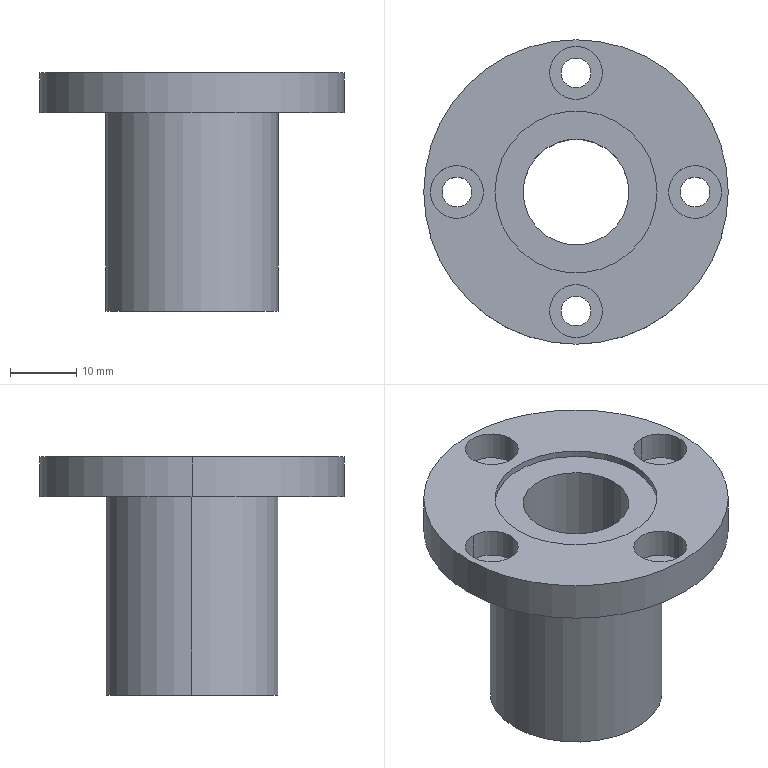Part | SolidWorks | features BaseBody 1 | 1 solid | 35 faces | box 46 x 46 x 36 mm | volume 17134 mm3 | cylinder 26 | plane 9 | commonest cylinder face diameters 4.5 x8 8 x8 24.5 x4 16 x2 26 x2 46 x2
STEP:
#1=CARTESIAN_POINT('',(13.,0.,-18.));
#2=VERTEX_POINT('',#1);
#3=CARTESIAN_POINT('',(-13.,0.,-18.));
#4=VERTEX_POINT('',#3);
#5=CARTESIAN_POINT('',(0.,0.,-18.));
#6=DIRECTION('',(0.,0.,1.));
#7=DIRECTION('',(1.,0.,0.));
#8=AXIS2_PLACEMENT_3D('',#5,#6,#7);
#9=CIRCLE('',#8,13.);
#10=EDGE_CURVE('',#2,#4,#9,.T.);
#11=ORIENTED_EDGE('',*,*,#10,.T.);
#12=CARTESIAN_POINT('',(-13.,0.,12.));
#13=VERTEX_POINT('',#12);
#14=CARTESIAN_POINT('',(-13.,0.,0.));
#15=DIRECTION('',(0.,0.,1.));
#16=VECTOR('',#15,1000.);
#17=LINE('',#14,#16);
#18=EDGE_CURVE('',#4,#13,#17,.T.);
#19=ORIENTED_EDGE('',*,*,#18,.T.);
#20=CARTESIAN_POINT('',(13.,0.,12.));
#21=VERTEX_POINT('',#20);
#22=CARTESIAN_POINT('',(0.,0.,12.));
#23=DIRECTION('',(0.,0.,-1.));
#24=DIRECTION('',(1.,0.,0.));
#25=AXIS2_PLACEMENT_3D('',#22,#23,#24);
#26=CIRCLE('',#25,13.);
#27=EDGE_CURVE('',#13,#21,#26,.T.);
#28=ORIENTED_EDGE('',*,*,#27,.T.);
#29=CARTESIAN_POINT('',(13.,0.,0.));
#30=DIRECTION('',(0.,0.,1.));
#31=VECTOR('',#30,1000.);
#32=LINE('',#29,#31);
#33=EDGE_CURVE('',#2,#21,#32,.T.);
#34=ORIENTED_EDGE('',*,*,#33,.F.);
#35=EDGE_LOOP('',(#11,#19,#28,#34));
#36=FACE_OUTER_BOUND('',#35,.T.);
#37=CARTESIAN_POINT('',(0.,0.,0.));
#38=DIRECTION('',(0.,0.,1.));
#39=DIRECTION('',(1.,0.,0.));
#40=AXIS2_PLACEMENT_3D('',#37,#38,#39);
#41=CYLINDRICAL_SURFACE('',#40,13.);
#42=ADVANCED_FACE('',(#36),#41,.T.);
#43=CARTESIAN_POINT('',(18.,-2.25,13.6));
#44=VERTEX_POINT('',#43);
#45=CARTESIAN_POINT('',(18.,2.25,13.6));
#46=VERTEX_POINT('',#45);
#47=CARTESIAN_POINT('',(18.,0.,13.6));
#48=DIRECTION('',(0.,0.,-1.));
#49=DIRECTION('',(0.,1.,0.));
#50=AXIS2_PLACEMENT_3D('',#47,#48,#49);
#51=CIRCLE('',#50,2.25);
#52=EDGE_CURVE('',#44,#46,#51,.T.);
#53=ORIENTED_EDGE('',*,*,#52,.F.);
#54=CARTESIAN_POINT('',(18.,-2.25,12.));
#55=VERTEX_POINT('',#54);
#56=CARTESIAN_POINT('',(18.,-2.25,13.6));
#57=DIRECTION('',(0.,0.,-1.));
#58=VECTOR('',#57,1000.);
#59=LINE('',#56,#58);
#60=EDGE_CURVE('',#44,#55,#59,.T.);
#61=ORIENTED_EDGE('',*,*,#60,.T.);
#62=CARTESIAN_POINT('',(18.,2.25,12.));
#63=VERTEX_POINT('',#62);
#64=CARTESIAN_POINT('',(18.,0.,12.));
#65=DIRECTION('',(0.,0.,1.));
#66=DIRECTION('',(0.,1.,0.));
#67=AXIS2_PLACEMENT_3D('',#64,#65,#66);
#68=CIRCLE('',#67,2.25);
#69=EDGE_CURVE('',#63,#55,#68,.T.);
#70=ORIENTED_EDGE('',*,*,#69,.F.);
#71=CARTESIAN_POINT('',(18.,2.25,13.6));
#72=DIRECTION('',(0.,0.,-1.));
#73=VECTOR('',#72,1000.);
#74=LINE('',#71,#73);
#75=EDGE_CURVE('',#46,#63,#74,.T.);
#76=ORIENTED_EDGE('',*,*,#75,.F.);
#77=EDGE_LOOP('',(#53,#61,#70,#76));
#78=FACE_OUTER_BOUND('',#77,.T.);
#79=CARTESIAN_POINT('',(18.,0.,13.6));
#80=DIRECTION('',(0.,0.,-1.));
#81=DIRECTION('',(0.,1.,0.));
#82=AXIS2_PLACEMENT_3D('',#79,#80,#81);
#83=CYLINDRICAL_SURFACE('',#82,2.25);
#84=ADVANCED_FACE('',(#78),#83,.F.);
#85=CARTESIAN_POINT('',(2.25,18.,13.6));
#86=VERTEX_POINT('',#85);
#87=CARTESIAN_POINT('',(-2.25,18.,13.6));
#88=VERTEX_POINT('',#87);
#89=CARTESIAN_POINT('',(0.,18.,13.6));
#90=DIRECTION('',(0.,0.,-1.));
#91=DIRECTION('',(-1.,0.,0.));
#92=AXIS2_PLACEMENT_3D('',#89,#90,#91);
#93=CIRCLE('',#92,2.25);
#94=EDGE_CURVE('',#86,#88,#93,.T.);
#95=ORIENTED_EDGE('',*,*,#94,.F.);
#96=CARTESIAN_POINT('',(2.25,18.,12.));
#97=VERTEX_POINT('',#96);
#98=CARTESIAN_POINT('',(2.25,18.,13.6));
#99=DIRECTION('',(0.,0.,-1.));
#100=VECTOR('',#99,1000.);
#101=LINE('',#98,#100);
#102=EDGE_CURVE('',#86,#97,#101,.T.);
#103=ORIENTED_EDGE('',*,*,#102,.T.);
#104=CARTESIAN_POINT('',(-2.25,18.,12.));
#105=VERTEX_POINT('',#104);
#106=CARTESIAN_POINT('',(0.,18.,12.));
#107=DIRECTION('',(0.,0.,1.));
#108=DIRECTION('',(-1.,0.,0.));
#109=AXIS2_PLACEMENT_3D('',#106,#107,#108);
#110=CIRCLE('',#109,2.25);
#111=EDGE_CURVE('',#105,#97,#110,.T.);
#112=ORIENTED_EDGE('',*,*,#111,.F.);
#113=CARTESIAN_POINT('',(-2.25,18.,13.6));
#114=DIRECTION('',(0.,0.,-1.));
#115=VECTOR('',#114,1000.);
#116=LINE('',#113,#115);
#117=EDGE_CURVE('',#88,#105,#116,.T.);
#118=ORIENTED_EDGE('',*,*,#117,.F.);
#119=EDGE_LOOP('',(#95,#103,#112,#118));
#120=FACE_OUTER_BOUND('',#119,.T.);
#121=CARTESIAN_POINT('',(0.,18.,13.6));
#122=DIRECTION('',(0.,0.,-1.));
#123=DIRECTION('',(-1.,0.,0.));
#124=AXIS2_PLACEMENT_3D('',#121,#122,#123);
#125=CYLINDRICAL_SURFACE('',#124,2.25);
#126=ADVANCED_FACE('',(#120),#125,.F.);
#127=CARTESIAN_POINT('',(-18.,-2.25,13.6));
#128=VERTEX_POINT('',#127);
#129=CARTESIAN_POINT('',(-18.,2.25,13.6));
#130=VERTEX_POINT('',#129);
#131=CARTESIAN_POINT('',(-18.,0.,13.6));
#132=DIRECTION('',(0.,0.,-1.));
#133=DIRECTION('',(0.,1.,0.));
#134=AXIS2_PLACEMENT_3D('',#131,#132,#133);
#135=CIRCLE('',#134,2.25);
#136=EDGE_CURVE('',#128,#130,#135,.T.);
#137=ORIENTED_EDGE('',*,*,#136,.F.);
#138=CARTESIAN_POINT('',(-18.,-2.25,12.));
#139=VERTEX_POINT('',#138);
#140=CARTESIAN_POINT('',(-18.,-2.25,13.6));
#141=DIRECTION('',(0.,0.,-1.));
#142=VECTOR('',#141,1000.);
#143=LINE('',#140,#142);
#144=EDGE_CURVE('',#128,#139,#143,.T.);
#145=ORIENTED_EDGE('',*,*,#144,.T.);
#146=CARTESIAN_POINT('',(-18.,2.25,12.));
#147=VERTEX_POINT('',#146);
#148=CARTESIAN_POINT('',(-18.,0.,12.));
#149=DIRECTION('',(0.,0.,1.));
#150=DIRECTION('',(0.,1.,0.));
#151=AXIS2_PLACEMENT_3D('',#148,#149,#150);
#152=CIRCLE('',#151,2.25);
#153=EDGE_CURVE('',#147,#139,#152,.T.);
#154=ORIENTED_EDGE('',*,*,#153,.F.);
#155=CARTESIAN_POINT('',(-18.,2.25,13.6));
#156=DIRECTION('',(0.,0.,-1.));
#157=VECTOR('',#156,1000.);
#158=LINE('',#155,#157);
#159=EDGE_CURVE('',#130,#147,#158,.T.);
#160=ORIENTED_EDGE('',*,*,#159,.F.);
#161=EDGE_LOOP('',(#137,#145,#154,#160));
#162=FACE_OUTER_BOUND('',#161,.T.);
#163=CARTESIAN_POINT('',(-18.,0.,13.6));
#164=DIRECTION('',(0.,0.,-1.));
#165=DIRECTION('',(0.,1.,0.));
#166=AXIS2_PLACEMENT_3D('',#163,#164,#165);
#167=CYLINDRICAL_SURFACE('',#166,2.25);
#168=ADVANCED_FACE('',(#162),#167,.F.);
#169=CARTESIAN_POINT('',(2.25,-18.,13.6));
#170=VERTEX_POINT('',#169);
#171=CARTESIAN_POINT('',(-2.25,-18.,13.6));
#172=VERTEX_POINT('',#171);
#173=CARTESIAN_POINT('',(0.,-18.,13.6));
#174=DIRECTION('',(0.,0.,-1.));
#175=DIRECTION('',(-1.,0.,0.));
#176=AXIS2_PLACEMENT_3D('',#173,#174,#175);
#177=CIRCLE('',#176,2.25);
#178=EDGE_CURVE('',#170,#172,#177,.T.);
#179=ORIENTED_EDGE('',*,*,#178,.F.);
#180=CARTESIAN_POINT('',(2.25,-18.,12.));
#181=VERTEX_POINT('',#180);
#182=CARTESIAN_POINT('',(2.25,-18.,13.6));
#183=DIRECTION('',(0.,0.,-1.));
#184=VECTOR('',#183,1000.);
#185=LINE('',#182,#184);
#186=EDGE_CURVE('',#170,#181,#185,.T.);
#187=ORIENTED_EDGE('',*,*,#186,.T.);
#188=CARTESIAN_POINT('',(-2.25,-18.,12.));
#189=VERTEX_POINT('',#188);
#190=CARTESIAN_POINT('',(0.,-18.,12.));
#191=DIRECTION('',(0.,0.,1.));
#192=DIRECTION('',(-1.,0.,0.));
#193=AXIS2_PLACEMENT_3D('',#190,#191,#192);
#194=CIRCLE('',#193,2.25);
#195=EDGE_CURVE('',#189,#181,#194,.T.);
#196=ORIENTED_EDGE('',*,*,#195,.F.);
#197=CARTESIAN_POINT('',(-2.25,-18.,13.6));
#198=DIRECTION('',(0.,0.,-1.));
#199=VECTOR('',#198,1000.);
#200=LINE('',#197,#199);
#201=EDGE_CURVE('',#172,#189,#200,.T.);
#202=ORIENTED_EDGE('',*,*,#201,.F.);
#203=EDGE_LOOP('',(#179,#187,#196,#202));
#204=FACE_OUTER_BOUND('',#203,.T.);
#205=CARTESIAN_POINT('',(0.,-18.,13.6));
#206=DIRECTION('',(0.,0.,-1.));
#207=DIRECTION('',(-1.,0.,0.));
#208=AXIS2_PLACEMENT_3D('',#205,#206,#207);
#209=CYLINDRICAL_SURFACE('',#208,2.25);
#210=ADVANCED_FACE('',(#204),#209,.F.);
#211=CARTESIAN_POINT('',(-23.,0.,18.));
#212=VERTEX_POINT('',#211);
#213=CARTESIAN_POINT('',(23.,0.,18.));
#214=VERTEX_POINT('',#213);
#215=CARTESIAN_POINT('',(0.,0.,18.));
#216=DIRECTION('',(0.,0.,-1.));
#217=DIRECTION('',(-1.,0.,0.));
#218=AXIS2_PLACEMENT_3D('',#215,#216,#217);
#219=CIRCLE('',#218,23.);
#220=EDGE_CURVE('',#212,#214,#219,.T.);
#221=ORIENTED_EDGE('',*,*,#220,.T.);
#222=CARTESIAN_POINT('',(23.,0.,12.));
#223=VERTEX_POINT('',#222);
#224=CARTESIAN_POINT('',(23.,0.,18.));
#225=DIRECTION('',(0.,0.,-1.));
#226=VECTOR('',#225,1000.);
#227=LINE('',#224,#226);
#228=EDGE_CURVE('',#214,#223,#227,.T.);
#229=ORIENTED_EDGE('',*,*,#228,.T.);
#230=CARTESIAN_POINT('',(-23.,0.,12.));
#231=VERTEX_POINT('',#230);
#232=CARTESIAN_POINT('',(0.,0.,12.));
#233=DIRECTION('',(0.,0.,-1.));
#234=DIRECTION('',(-1.,0.,0.));
#235=AXIS2_PLACEMENT_3D('',#232,#233,#234);
#236=CIRCLE('',#235,23.);
#237=EDGE_CURVE('',#231,#223,#236,.T.);
#238=ORIENTED_EDGE('',*,*,#237,.F.);
#239=CARTESIAN_POINT('',(-23.,0.,18.));
#240=DIRECTION('',(0.,0.,-1.));
#241=VECTOR('',#240,1000.);
#242=LINE('',#239,#241);
#243=EDGE_CURVE('',#212,#231,#242,.T.);
#244=ORIENTED_EDGE('',*,*,#243,.F.);
#245=EDGE_LOOP('',(#221,#229,#238,#244));
#246=FACE_OUTER_BOUND('',#245,.T.);
#247=CARTESIAN_POINT('',(0.,0.,18.));
#248=DIRECTION('',(0.,0.,-1.));
#249=DIRECTION('',(-1.,0.,0.));
#250=AXIS2_PLACEMENT_3D('',#247,#248,#249);
#251=CYLINDRICAL_SURFACE('',#250,23.);
#252=ADVANCED_FACE('',(#246),#251,.T.);
#253=CARTESIAN_POINT('',(-12.25,0.,-18.));
#254=VERTEX_POINT('',#253);
#255=CARTESIAN_POINT('',(12.25,0.,-18.));
#256=VERTEX_POINT('',#255);
#257=CARTESIAN_POINT('',(0.,0.,-18.));
#258=DIRECTION('',(0.,0.,1.));
#259=DIRECTION('',(1.,0.,0.));
#260=AXIS2_PLACEMENT_3D('',#257,#258,#259);
#261=CIRCLE('',#260,12.25);
#262=EDGE_CURVE('',#254,#256,#261,.T.);
#263=ORIENTED_EDGE('',*,*,#262,.F.);
#264=CARTESIAN_POINT('',(-12.25,0.,-17.));
#265=VERTEX_POINT('',#264);
#266=CARTESIAN_POINT('',(-12.25,0.,0.));
#267=DIRECTION('',(0.,0.,1.));
#268=VECTOR('',#267,1000.);
#269=LINE('',#266,#268);
#270=EDGE_CURVE('',#254,#265,#269,.T.);
#271=ORIENTED_EDGE('',*,*,#270,.T.);
#272=CARTESIAN_POINT('',(12.25,0.,-17.));
#273=VERTEX_POINT('',#272);
#274=CARTESIAN_POINT('',(0.,0.,-17.));
#275=DIRECTION('',(0.,0.,-1.));
#276=DIRECTION('',(1.,0.,0.));
#277=AXIS2_PLACEMENT_3D('',#274,#275,#276);
#278=CIRCLE('',#277,12.25);
#279=EDGE_CURVE('',#273,#265,#278,.T.);
#280=ORIENTED_EDGE('',*,*,#279,.F.);
#281=CARTESIAN_POINT('',(12.25,0.,0.));
#282=DIRECTION('',(0.,0.,1.));
#283=VECTOR('',#282,1000.);
#284=LINE('',#281,#283);
#285=EDGE_CURVE('',#256,#273,#284,.T.);
#286=ORIENTED_EDGE('',*,*,#285,.F.);
#287=EDGE_LOOP('',(#263,#271,#280,#286));
#288=FACE_OUTER_BOUND('',#287,.T.);
#289=CARTESIAN_POINT('',(0.,0.,0.));
#290=DIRECTION('',(0.,0.,1.));
#291=DIRECTION('',(1.,0.,0.));
#292=AXIS2_PLACEMENT_3D('',#289,#290,#291);
#293=CYLINDRICAL_SURFACE('',#292,12.25);
#294=ADVANCED_FACE('',(#288),#293,.F.);
#295=CARTESIAN_POINT('',(18.,4.,18.));
#296=VERTEX_POINT('',#295);
#297=CARTESIAN_POINT('',(18.,-4.,18.));
#298=VERTEX_POINT('',#297);
#299=CARTESIAN_POINT('',(18.,0.,18.));
#300=DIRECTION('',(0.,0.,1.));
#301=DIRECTION('',(0.,1.,0.));
#302=AXIS2_PLACEMENT_3D('',#299,#300,#301);
#303=CIRCLE('',#302,4.);
#304=EDGE_CURVE('',#296,#298,#303,.T.);
#305=ORIENTED_EDGE('',*,*,#304,.T.);
#306=CARTESIAN_POINT('',(18.,-4.,13.6));
#307=VERTEX_POINT('',#306);
#308=CARTESIAN_POINT('',(18.,-4.,18.));
#309=DIRECTION('',(0.,0.,-1.));
#310=VECTOR('',#309,1000.);
#311=LINE('',#308,#310);
#312=EDGE_CURVE('',#298,#307,#311,.T.);
#313=ORIENTED_EDGE('',*,*,#312,.T.);
#314=CARTESIAN_POINT('',(18.,4.,13.6));
#315=VERTEX_POINT('',#314);
#316=CARTESIAN_POINT('',(18.,0.,13.6));
#317=DIRECTION('',(0.,0.,-1.));
#318=DIRECTION('',(0.,1.,0.));
#319=AXIS2_PLACEMENT_3D('',#316,#317,#318);
#320=CIRCLE('',#319,4.);
#321=EDGE_CURVE('',#307,#315,#320,.T.);
#322=ORIENTED_EDGE('',*,*,#321,.T.);
#323=CARTESIAN_POINT('',(18.,4.,18.));
#324=DIRECTION('',(0.,0.,-1.));
#325=VECTOR('',#324,1000.);
#326=LINE('',#323,#325);
#327=EDGE_CURVE('',#296,#315,#326,.T.);
#328=ORIENTED_EDGE('',*,*,#327,.F.);
#329=EDGE_LOOP('',(#305,#313,#322,#328));
#330=FACE_OUTER_BOUND('',#329,.T.);
#331=CARTESIAN_POINT('',(18.,0.,18.));
#332=DIRECTION('',(0.,0.,-1.));
#333=DIRECTION('',(0.,1.,0.));
#334=AXIS2_PLACEMENT_3D('',#331,#332,#333);
#335=CYLINDRICAL_SURFACE('',#334,4.);
#336=ADVANCED_FACE('',(#330),#335,.F.);
#337=CARTESIAN_POINT('',(-4.,18.,18.));
#338=VERTEX_POINT('',#337);
#339=CARTESIAN_POINT('',(4.,18.,18.));
#340=VERTEX_POINT('',#339);
#341=CARTESIAN_POINT('',(0.,18.,18.));
#342=DIRECTION('',(0.,0.,1.));
#343=DIRECTION('',(-1.,0.,0.));
#344=AXIS2_PLACEMENT_3D('',#341,#342,#343);
#345=CIRCLE('',#344,4.);
#346=EDGE_CURVE('',#338,#340,#345,.T.);
#347=ORIENTED_EDGE('',*,*,#346,.T.);
#348=CARTESIAN_POINT('',(4.,18.,13.6));
#349=VERTEX_POINT('',#348);
#350=CARTESIAN_POINT('',(4.,18.,18.));
#351=DIRECTION('',(0.,0.,-1.));
#352=VECTOR('',#351,1000.);
#353=LINE('',#350,#352);
#354=EDGE_CURVE('',#340,#349,#353,.T.);
#355=ORIENTED_EDGE('',*,*,#354,.T.);
#356=CARTESIAN_POINT('',(-4.,18.,13.6));
#357=VERTEX_POINT('',#356);
#358=CARTESIAN_POINT('',(0.,18.,13.6));
#359=DIRECTION('',(0.,0.,-1.));
#360=DIRECTION('',(-1.,0.,0.));
#361=AXIS2_PLACEMENT_3D('',#358,#359,#360);
#362=CIRCLE('',#361,4.);
#363=EDGE_CURVE('',#349,#357,#362,.T.);
#364=ORIENTED_EDGE('',*,*,#363,.T.);
#365=CARTESIAN_POINT('',(-4.,18.,18.));
#366=DIRECTION('',(0.,0.,-1.));
#367=VECTOR('',#366,1000.);
#368=LINE('',#365,#367);
#369=EDGE_CURVE('',#338,#357,#368,.T.);
#370=ORIENTED_EDGE('',*,*,#369,.F.);
#371=EDGE_LOOP('',(#347,#355,#364,#370));
#372=FACE_OUTER_BOUND('',#371,.T.);
#373=CARTESIAN_POINT('',(0.,18.,18.));
#374=DIRECTION('',(0.,0.,-1.));
#375=DIRECTION('',(-1.,0.,0.));
#376=AXIS2_PLACEMENT_3D('',#373,#374,#375);
#377=CYLINDRICAL_SURFACE('',#376,4.);
#378=ADVANCED_FACE('',(#372),#377,.F.);
#379=CARTESIAN_POINT('',(-18.,4.,18.));
#380=VERTEX_POINT('',#379);
#381=CARTESIAN_POINT('',(-18.,-4.,18.));
#382=VERTEX_POINT('',#381);
#383=CARTESIAN_POINT('',(-18.,0.,18.));
#384=DIRECTION('',(0.,0.,1.));
#385=DIRECTION('',(0.,1.,0.));
#386=AXIS2_PLACEMENT_3D('',#383,#384,#385);
#387=CIRCLE('',#386,4.);
#388=EDGE_CURVE('',#380,#382,#387,.T.);
#389=ORIENTED_EDGE('',*,*,#388,.T.);
#390=CARTESIAN_POINT('',(-18.,-4.,13.6));
#391=VERTEX_POINT('',#390);
#392=CARTESIAN_POINT('',(-18.,-4.,18.));
#393=DIRECTION('',(0.,0.,-1.));
#394=VECTOR('',#393,1000.);
#395=LINE('',#392,#394);
#396=EDGE_CURVE('',#382,#391,#395,.T.);
#397=ORIENTED_EDGE('',*,*,#396,.T.);
#398=CARTESIAN_POINT('',(-18.,4.,13.6));
#399=VERTEX_POINT('',#398);
#400=CARTESIAN_POINT('',(-18.,0.,13.6));
#401=DIRECTION('',(0.,0.,-1.));
#402=DIRECTION('',(0.,1.,0.));
#403=AXIS2_PLACEMENT_3D('',#400,#401,#402);
#404=CIRCLE('',#403,4.);
#405=EDGE_CURVE('',#391,#399,#404,.T.);
#406=ORIENTED_EDGE('',*,*,#405,.T.);
#407=CARTESIAN_POINT('',(-18.,4.,18.));
#408=DIRECTION('',(0.,0.,-1.));
#409=VECTOR('',#408,1000.);
#410=LINE('',#407,#409);
#411=EDGE_CURVE('',#380,#399,#410,.T.);
#412=ORIENTED_EDGE('',*,*,#411,.F.);
#413=EDGE_LOOP('',(#389,#397,#406,#412));
#414=FACE_OUTER_BOUND('',#413,.T.);
#415=CARTESIAN_POINT('',(-18.,0.,18.));
#416=DIRECTION('',(0.,0.,-1.));
#417=DIRECTION('',(0.,1.,0.));
#418=AXIS2_PLACEMENT_3D('',#415,#416,#417);
#419=CYLINDRICAL_SURFACE('',#418,4.);
#420=ADVANCED_FACE('',(#414),#419,.F.);
#421=CARTESIAN_POINT('',(-4.,-18.,18.));
#422=VERTEX_POINT('',#421);
#423=CARTESIAN_POINT('',(4.,-18.,18.));
#424=VERTEX_POINT('',#423);
#425=CARTESIAN_POINT('',(0.,-18.,18.));
#426=DIRECTION('',(0.,0.,1.));
#427=DIRECTION('',(-1.,0.,0.));
#428=AXIS2_PLACEMENT_3D('',#425,#426,#427);
#429=CIRCLE('',#428,4.);
#430=EDGE_CURVE('',#422,#424,#429,.T.);
#431=ORIENTED_EDGE('',*,*,#430,.T.);
#432=CARTESIAN_POINT('',(4.,-18.,13.6));
#433=VERTEX_POINT('',#432);
#434=CARTESIAN_POINT('',(4.,-18.,18.));
#435=DIRECTION('',(0.,0.,-1.));
#436=VECTOR('',#435,1000.);
#437=LINE('',#434,#436);
#438=EDGE_CURVE('',#424,#433,#437,.T.);
#439=ORIENTED_EDGE('',*,*,#438,.T.);
#440=CARTESIAN_POINT('',(-4.,-18.,13.6));
#441=VERTEX_POINT('',#440);
#442=CARTESIAN_POINT('',(0.,-18.,13.6));
#443=DIRECTION('',(0.,0.,-1.));
#444=DIRECTION('',(-1.,0.,0.));
#445=AXIS2_PLACEMENT_3D('',#442,#443,#444);
#446=CIRCLE('',#445,4.);
#447=EDGE_CURVE('',#433,#441,#446,.T.);
#448=ORIENTED_EDGE('',*,*,#447,.T.);
#449=CARTESIAN_POINT('',(-4.,-18.,18.));
#450=DIRECTION('',(0.,0.,-1.));
#451=VECTOR('',#450,1000.);
#452=LINE('',#449,#451);
#453=EDGE_CURVE('',#422,#441,#452,.T.);
#454=ORIENTED_EDGE('',*,*,#453,.F.);
#455=EDGE_LOOP('',(#431,#439,#448,#454));
#456=FACE_OUTER_BOUND('',#455,.T.);
#457=CARTESIAN_POINT('',(0.,-18.,18.));
#458=DIRECTION('',(0.,0.,-1.));
#459=DIRECTION('',(-1.,0.,0.));
#460=AXIS2_PLACEMENT_3D('',#457,#458,#459);
#461=CYLINDRICAL_SURFACE('',#460,4.);
#462=ADVANCED_FACE('',(#456),#461,.F.);
#463=CARTESIAN_POINT('',(-12.25,0.,17.));
#464=VERTEX_POINT('',#463);
#465=CARTESIAN_POINT('',(12.25,0.,17.));
#466=VERTEX_POINT('',#465);
#467=CARTESIAN_POINT('',(0.,0.,17.));
#468=DIRECTION('',(0.,0.,1.));
#469=DIRECTION('',(1.,0.,0.));
#470=AXIS2_PLACEMENT_3D('',#467,#468,#469);
#471=CIRCLE('',#470,12.25);
#472=EDGE_CURVE('',#464,#466,#471,.T.);
#473=ORIENTED_EDGE('',*,*,#472,.F.);
#474=CARTESIAN_POINT('',(-12.25,0.,18.));
#475=VERTEX_POINT('',#474);
#476=CARTESIAN_POINT('',(-12.25,0.,0.));
#477=DIRECTION('',(0.,0.,1.));
#478=VECTOR('',#477,1000.);
#479=LINE('',#476,#478);
#480=EDGE_CURVE('',#464,#475,#479,.T.);
#481=ORIENTED_EDGE('',*,*,#480,.T.);
#482=CARTESIAN_POINT('',(12.25,0.,18.));
#483=VERTEX_POINT('',#482);
#484=CARTESIAN_POINT('',(0.,0.,18.));
#485=DIRECTION('',(0.,0.,1.));
#486=DIRECTION('',(1.,0.,0.));
#487=AXIS2_PLACEMENT_3D('',#484,#485,#486);
#488=CIRCLE('',#487,12.25);
#489=EDGE_CURVE('',#475,#483,#488,.T.);
#490=ORIENTED_EDGE('',*,*,#489,.T.);
#491=CARTESIAN_POINT('',(12.25,0.,0.));
#492=DIRECTION('',(0.,0.,1.));
#493=VECTOR('',#492,1000.);
#494=LINE('',#491,#493);
#495=EDGE_CURVE('',#466,#483,#494,.T.);
#496=ORIENTED_EDGE('',*,*,#495,.F.);
#497=EDGE_LOOP('',(#473,#481,#490,#496));
#498=FACE_OUTER_BOUND('',#497,.T.);
#499=CARTESIAN_POINT('',(0.,0.,0.));
#500=DIRECTION('',(0.,0.,1.));
#501=DIRECTION('',(1.,0.,0.));
#502=AXIS2_PLACEMENT_3D('',#499,#500,#501);
#503=CYLINDRICAL_SURFACE('',#502,12.25);
#504=ADVANCED_FACE('',(#498),#503,.F.);
#505=CARTESIAN_POINT('',(-8.,0.,-17.));
#506=VERTEX_POINT('',#505);
#507=CARTESIAN_POINT('',(8.,0.,-17.));
#508=VERTEX_POINT('',#507);
#509=CARTESIAN_POINT('',(0.,0.,-17.));
#510=DIRECTION('',(0.,0.,1.));
#511=DIRECTION('',(1.,0.,0.));
#512=AXIS2_PLACEMENT_3D('',#509,#510,#511);
#513=CIRCLE('',#512,8.);
#514=EDGE_CURVE('',#506,#508,#513,.T.);
#515=ORIENTED_EDGE('',*,*,#514,.F.);
#516=CARTESIAN_POINT('',(-8.,0.,17.));
#517=VERTEX_POINT('',#516);
#518=CARTESIAN_POINT('',(-8.,0.,0.));
#519=DIRECTION('',(0.,0.,1.));
#520=VECTOR('',#519,1000.);
#521=LINE('',#518,#520);
#522=EDGE_CURVE('',#506,#517,#521,.T.);
#523=ORIENTED_EDGE('',*,*,#522,.T.);
#524=CARTESIAN_POINT('',(8.,0.,17.));
#525=VERTEX_POINT('',#524);
#526=CARTESIAN_POINT('',(0.,0.,17.));
#527=DIRECTION('',(0.,0.,-1.));
#528=DIRECTION('',(1.,0.,0.));
#529=AXIS2_PLACEMENT_3D('',#526,#527,#528);
#530=CIRCLE('',#529,8.);
#531=EDGE_CURVE('',#525,#517,#530,.T.);
#532=ORIENTED_EDGE('',*,*,#531,.F.);
#533=CARTESIAN_POINT('',(8.,0.,0.));
#534=DIRECTION('',(0.,0.,1.));
#535=VECTOR('',#534,1000.);
#536=LINE('',#533,#535);
#537=EDGE_CURVE('',#508,#525,#536,.T.);
#538=ORIENTED_EDGE('',*,*,#537,.F.);
#539=EDGE_LOOP('',(#515,#523,#532,#538));
#540=FACE_OUTER_BOUND('',#539,.T.);
#541=CARTESIAN_POINT('',(0.,0.,0.));
#542=DIRECTION('',(0.,0.,1.));
#543=DIRECTION('',(1.,0.,0.));
#544=AXIS2_PLACEMENT_3D('',#541,#542,#543);
#545=CYLINDRICAL_SURFACE('',#544,8.);
#546=ADVANCED_FACE('',(#540),#545,.F.);
#547=ORIENTED_EDGE('',*,*,#18,.F.);
#548=CARTESIAN_POINT('',(0.,0.,-18.));
#549=DIRECTION('',(0.,0.,1.));
#550=DIRECTION('',(1.,0.,0.));
#551=AXIS2_PLACEMENT_3D('',#548,#549,#550);
#552=CIRCLE('',#551,13.);
#553=EDGE_CURVE('',#4,#2,#552,.T.);
#554=ORIENTED_EDGE('',*,*,#553,.T.);
#555=ORIENTED_EDGE('',*,*,#33,.T.);
#556=CARTESIAN_POINT('',(0.,0.,12.));
#557=DIRECTION('',(0.,0.,-1.));
#558=DIRECTION('',(1.,0.,0.));
#559=AXIS2_PLACEMENT_3D('',#556,#557,#558);
#560=CIRCLE('',#559,13.);
#561=EDGE_CURVE('',#21,#13,#560,.T.);
#562=ORIENTED_EDGE('',*,*,#561,.T.);
#563=EDGE_LOOP('',(#547,#554,#555,#562));
#564=FACE_OUTER_BOUND('',#563,.T.);
#565=CARTESIAN_POINT('',(0.,0.,0.));
#566=DIRECTION('',(0.,0.,1.));
#567=DIRECTION('',(1.,0.,0.));
#568=AXIS2_PLACEMENT_3D('',#565,#566,#567);
#569=CYLINDRICAL_SURFACE('',#568,13.);
#570=ADVANCED_FACE('',(#564),#569,.T.);
#571=ORIENTED_EDGE('',*,*,#561,.F.);
#572=ORIENTED_EDGE('',*,*,#27,.F.);
#573=EDGE_LOOP('',(#571,#572));
#574=FACE_BOUND('',#573,.T.);
#575=ORIENTED_EDGE('',*,*,#69,.T.);
#576=CARTESIAN_POINT('',(18.,0.,12.));
#577=DIRECTION('',(0.,0.,1.));
#578=DIRECTION('',(0.,1.,0.));
#579=AXIS2_PLACEMENT_3D('',#576,#577,#578);
#580=CIRCLE('',#579,2.25);
#581=EDGE_CURVE('',#55,#63,#580,.T.);
#582=ORIENTED_EDGE('',*,*,#581,.T.);
#583=EDGE_LOOP('',(#575,#582));
#584=FACE_BOUND('',#583,.T.);
#585=ORIENTED_EDGE('',*,*,#111,.T.);
#586=CARTESIAN_POINT('',(0.,18.,12.));
#587=DIRECTION('',(0.,0.,1.));
#588=DIRECTION('',(-1.,0.,0.));
#589=AXIS2_PLACEMENT_3D('',#586,#587,#588);
#590=CIRCLE('',#589,2.25);
#591=EDGE_CURVE('',#97,#105,#590,.T.);
#592=ORIENTED_EDGE('',*,*,#591,.T.);
#593=EDGE_LOOP('',(#585,#592));
#594=FACE_BOUND('',#593,.T.);
#595=ORIENTED_EDGE('',*,*,#153,.T.);
#596=CARTESIAN_POINT('',(-18.,0.,12.));
#597=DIRECTION('',(0.,0.,1.));
#598=DIRECTION('',(0.,1.,0.));
#599=AXIS2_PLACEMENT_3D('',#596,#597,#598);
#600=CIRCLE('',#599,2.25);
#601=EDGE_CURVE('',#139,#147,#600,.T.);
#602=ORIENTED_EDGE('',*,*,#601,.T.);
#603=EDGE_LOOP('',(#595,#602));
#604=FACE_BOUND('',#603,.T.);
#605=ORIENTED_EDGE('',*,*,#195,.T.);
#606=CARTESIAN_POINT('',(0.,-18.,12.));
#607=DIRECTION('',(0.,0.,1.));
#608=DIRECTION('',(-1.,0.,0.));
#609=AXIS2_PLACEMENT_3D('',#606,#607,#608);
#610=CIRCLE('',#609,2.25);
#611=EDGE_CURVE('',#181,#189,#610,.T.);
#612=ORIENTED_EDGE('',*,*,#611,.T.);
#613=EDGE_LOOP('',(#605,#612));
#614=FACE_BOUND('',#613,.T.);
#615=ORIENTED_EDGE('',*,*,#237,.T.);
#616=CARTESIAN_POINT('',(0.,0.,12.));
#617=DIRECTION('',(0.,0.,-1.));
#618=DIRECTION('',(-1.,0.,0.));
#619=AXIS2_PLACEMENT_3D('',#616,#617,#618);
#620=CIRCLE('',#619,23.);
#621=EDGE_CURVE('',#223,#231,#620,.T.);
#622=ORIENTED_EDGE('',*,*,#621,.T.);
#623=EDGE_LOOP('',(#615,#622));
#624=FACE_OUTER_BOUND('',#623,.T.);
#625=CARTESIAN_POINT('',(0.,0.,12.));
#626=DIRECTION('',(0.,0.,-1.));
#627=DIRECTION('',(-1.,0.,0.));
#628=AXIS2_PLACEMENT_3D('',#625,#626,#627);
#629=PLANE('',#628);
#630=ADVANCED_FACE('',(#574,#584,#594,#604,#614,#624),#629,.T.);
#631=CARTESIAN_POINT('',(0.,0.,-18.));
#632=DIRECTION('',(0.,0.,1.));
#633=DIRECTION('',(1.,0.,0.));
#634=AXIS2_PLACEMENT_3D('',#631,#632,#633);
#635=CIRCLE('',#634,12.25);
#636=EDGE_CURVE('',#256,#254,#635,.T.);
#637=ORIENTED_EDGE('',*,*,#636,.T.);
#638=ORIENTED_EDGE('',*,*,#262,.T.);
#639=EDGE_LOOP('',(#637,#638));
#640=FACE_BOUND('',#639,.T.);
#641=ORIENTED_EDGE('',*,*,#10,.F.);
#642=ORIENTED_EDGE('',*,*,#553,.F.);
#643=EDGE_LOOP('',(#641,#642));
#644=FACE_OUTER_BOUND('',#643,.T.);
#645=CARTESIAN_POINT('',(0.,0.,-18.));
#646=DIRECTION('',(0.,0.,-1.));
#647=DIRECTION('',(-1.,0.,0.));
#648=AXIS2_PLACEMENT_3D('',#645,#646,#647);
#649=PLANE('',#648);
#650=ADVANCED_FACE('',(#640,#644),#649,.T.);
#651=ORIENTED_EDGE('',*,*,#60,.F.);
#652=CARTESIAN_POINT('',(18.,0.,13.6));
#653=DIRECTION('',(0.,0.,-1.));
#654=DIRECTION('',(0.,1.,0.));
#655=AXIS2_PLACEMENT_3D('',#652,#653,#654);
#656=CIRCLE('',#655,2.25);
#657=EDGE_CURVE('',#46,#44,#656,.T.);
#658=ORIENTED_EDGE('',*,*,#657,.F.);
#659=ORIENTED_EDGE('',*,*,#75,.T.);
#660=ORIENTED_EDGE('',*,*,#581,.F.);
#661=EDGE_LOOP('',(#651,#658,#659,#660));
#662=FACE_OUTER_BOUND('',#661,.T.);
#663=CARTESIAN_POINT('',(18.,0.,13.6));
#664=DIRECTION('',(0.,0.,-1.));
#665=DIRECTION('',(0.,1.,0.));
#666=AXIS2_PLACEMENT_3D('',#663,#664,#665);
#667=CYLINDRICAL_SURFACE('',#666,2.25);
#668=ADVANCED_FACE('',(#662),#667,.F.);
#669=ORIENTED_EDGE('',*,*,#102,.F.);
#670=CARTESIAN_POINT('',(0.,18.,13.6));
#671=DIRECTION('',(0.,0.,-1.));
#672=DIRECTION('',(-1.,0.,0.));
#673=AXIS2_PLACEMENT_3D('',#670,#671,#672);
#674=CIRCLE('',#673,2.25);
#675=EDGE_CURVE('',#88,#86,#674,.T.);
#676=ORIENTED_EDGE('',*,*,#675,.F.);
#677=ORIENTED_EDGE('',*,*,#117,.T.);
#678=ORIENTED_EDGE('',*,*,#591,.F.);
#679=EDGE_LOOP('',(#669,#676,#677,#678));
#680=FACE_OUTER_BOUND('',#679,.T.);
#681=CARTESIAN_POINT('',(0.,18.,13.6));
#682=DIRECTION('',(0.,0.,-1.));
#683=DIRECTION('',(-1.,0.,0.));
#684=AXIS2_PLACEMENT_3D('',#681,#682,#683);
#685=CYLINDRICAL_SURFACE('',#684,2.25);
#686=ADVANCED_FACE('',(#680),#685,.F.);
#687=ORIENTED_EDGE('',*,*,#144,.F.);
#688=CARTESIAN_POINT('',(-18.,0.,13.6));
#689=DIRECTION('',(0.,0.,-1.));
#690=DIRECTION('',(0.,1.,0.));
#691=AXIS2_PLACEMENT_3D('',#688,#689,#690);
#692=CIRCLE('',#691,2.25);
#693=EDGE_CURVE('',#130,#128,#692,.T.);
#694=ORIENTED_EDGE('',*,*,#693,.F.);
#695=ORIENTED_EDGE('',*,*,#159,.T.);
#696=ORIENTED_EDGE('',*,*,#601,.F.);
#697=EDGE_LOOP('',(#687,#694,#695,#696));
#698=FACE_OUTER_BOUND('',#697,.T.);
#699=CARTESIAN_POINT('',(-18.,0.,13.6));
#700=DIRECTION('',(0.,0.,-1.));
#701=DIRECTION('',(0.,1.,0.));
#702=AXIS2_PLACEMENT_3D('',#699,#700,#701);
#703=CYLINDRICAL_SURFACE('',#702,2.25);
#704=ADVANCED_FACE('',(#698),#703,.F.);
#705=ORIENTED_EDGE('',*,*,#186,.F.);
#706=CARTESIAN_POINT('',(0.,-18.,13.6));
#707=DIRECTION('',(0.,0.,-1.));
#708=DIRECTION('',(-1.,0.,0.));
#709=AXIS2_PLACEMENT_3D('',#706,#707,#708);
#710=CIRCLE('',#709,2.25);
#711=EDGE_CURVE('',#172,#170,#710,.T.);
#712=ORIENTED_EDGE('',*,*,#711,.F.);
#713=ORIENTED_EDGE('',*,*,#201,.T.);
#714=ORIENTED_EDGE('',*,*,#611,.F.);
#715=EDGE_LOOP('',(#705,#712,#713,#714));
#716=FACE_OUTER_BOUND('',#715,.T.);
#717=CARTESIAN_POINT('',(0.,-18.,13.6));
#718=DIRECTION('',(0.,0.,-1.));
#719=DIRECTION('',(-1.,0.,0.));
#720=AXIS2_PLACEMENT_3D('',#717,#718,#719);
#721=CYLINDRICAL_SURFACE('',#720,2.25);
#722=ADVANCED_FACE('',(#716),#721,.F.);
#723=ORIENTED_EDGE('',*,*,#228,.F.);
#724=CARTESIAN_POINT('',(0.,0.,18.));
#725=DIRECTION('',(0.,0.,-1.));
#726=DIRECTION('',(-1.,0.,0.));
#727=AXIS2_PLACEMENT_3D('',#724,#725,#726);
#728=CIRCLE('',#727,23.);
#729=EDGE_CURVE('',#214,#212,#728,.T.);
#730=ORIENTED_EDGE('',*,*,#729,.T.);
#731=ORIENTED_EDGE('',*,*,#243,.T.);
#732=ORIENTED_EDGE('',*,*,#621,.F.);
#733=EDGE_LOOP('',(#723,#730,#731,#732));
#734=FACE_OUTER_BOUND('',#733,.T.);
#735=CARTESIAN_POINT('',(0.,0.,18.));
#736=DIRECTION('',(0.,0.,-1.));
#737=DIRECTION('',(-1.,0.,0.));
#738=AXIS2_PLACEMENT_3D('',#735,#736,#737);
#739=CYLINDRICAL_SURFACE('',#738,23.);
#740=ADVANCED_FACE('',(#734),#739,.T.);
#741=ORIENTED_EDGE('',*,*,#270,.F.);
#742=ORIENTED_EDGE('',*,*,#636,.F.);
#743=ORIENTED_EDGE('',*,*,#285,.T.);
#744=CARTESIAN_POINT('',(0.,0.,-17.));
#745=DIRECTION('',(0.,0.,-1.));
#746=DIRECTION('',(1.,0.,0.));
#747=AXIS2_PLACEMENT_3D('',#744,#745,#746);
#748=CIRCLE('',#747,12.25);
#749=EDGE_CURVE('',#265,#273,#748,.T.);
#750=ORIENTED_EDGE('',*,*,#749,.F.);
#751=EDGE_LOOP('',(#741,#742,#743,#750));
#752=FACE_OUTER_BOUND('',#751,.T.);
#753=CARTESIAN_POINT('',(0.,0.,0.));
#754=DIRECTION('',(0.,0.,1.));
#755=DIRECTION('',(1.,0.,0.));
#756=AXIS2_PLACEMENT_3D('',#753,#754,#755);
#757=CYLINDRICAL_SURFACE('',#756,12.25);
#758=ADVANCED_FACE('',(#752),#757,.F.);
#759=ORIENTED_EDGE('',*,*,#657,.T.);
#760=ORIENTED_EDGE('',*,*,#52,.T.);
#761=EDGE_LOOP('',(#759,#760));
#762=FACE_BOUND('',#761,.T.);
#763=CARTESIAN_POINT('',(18.,0.,13.6));
#764=DIRECTION('',(0.,0.,-1.));
#765=DIRECTION('',(0.,1.,0.));
#766=AXIS2_PLACEMENT_3D('',#763,#764,#765);
#767=CIRCLE('',#766,4.);
#768=EDGE_CURVE('',#315,#307,#767,.T.);
#769=ORIENTED_EDGE('',*,*,#768,.F.);
#770=ORIENTED_EDGE('',*,*,#321,.F.);
#771=EDGE_LOOP('',(#769,#770));
#772=FACE_OUTER_BOUND('',#771,.T.);
#773=CARTESIAN_POINT('',(14.,4.08,13.6));
#774=DIRECTION('',(0.,0.,-1.));
#775=DIRECTION('',(1.,0.,0.));
#776=AXIS2_PLACEMENT_3D('',#773,#774,#775);
#777=PLANE('',#776);
#778=ADVANCED_FACE('',(#762,#772),#777,.F.);
#779=ORIENTED_EDGE('',*,*,#675,.T.);
#780=ORIENTED_EDGE('',*,*,#94,.T.);
#781=EDGE_LOOP('',(#779,#780));
#782=FACE_BOUND('',#781,.T.);
#783=CARTESIAN_POINT('',(0.,18.,13.6));
#784=DIRECTION('',(0.,0.,-1.));
#785=DIRECTION('',(-1.,0.,0.));
#786=AXIS2_PLACEMENT_3D('',#783,#784,#785);
#787=CIRCLE('',#786,4.);
#788=EDGE_CURVE('',#357,#349,#787,.T.);
#789=ORIENTED_EDGE('',*,*,#788,.F.);
#790=ORIENTED_EDGE('',*,*,#363,.F.);
#791=EDGE_LOOP('',(#789,#790));
#792=FACE_OUTER_BOUND('',#791,.T.);
#793=CARTESIAN_POINT('',(-4.08,14.,13.6));
#794=DIRECTION('',(0.,0.,-1.));
#795=DIRECTION('',(0.,1.,0.));
#796=AXIS2_PLACEMENT_3D('',#793,#794,#795);
#797=PLANE('',#796);
#798=ADVANCED_FACE('',(#782,#792),#797,.F.);
#799=ORIENTED_EDGE('',*,*,#693,.T.);
#800=ORIENTED_EDGE('',*,*,#136,.T.);
#801=EDGE_LOOP('',(#799,#800));
#802=FACE_BOUND('',#801,.T.);
#803=CARTESIAN_POINT('',(-18.,0.,13.6));
#804=DIRECTION('',(0.,0.,-1.));
#805=DIRECTION('',(0.,1.,0.));
#806=AXIS2_PLACEMENT_3D('',#803,#804,#805);
#807=CIRCLE('',#806,4.);
#808=EDGE_CURVE('',#399,#391,#807,.T.);
#809=ORIENTED_EDGE('',*,*,#808,.F.);
#810=ORIENTED_EDGE('',*,*,#405,.F.);
#811=EDGE_LOOP('',(#809,#810));
#812=FACE_OUTER_BOUND('',#811,.T.);
#813=CARTESIAN_POINT('',(-14.,-4.08,13.6));
#814=DIRECTION('',(0.,0.,-1.));
#815=DIRECTION('',(-1.,0.,0.));
#816=AXIS2_PLACEMENT_3D('',#813,#814,#815);
#817=PLANE('',#816);
#818=ADVANCED_FACE('',(#802,#812),#817,.F.);
#819=ORIENTED_EDGE('',*,*,#711,.T.);
#820=ORIENTED_EDGE('',*,*,#178,.T.);
#821=EDGE_LOOP('',(#819,#820));
#822=FACE_BOUND('',#821,.T.);
#823=CARTESIAN_POINT('',(0.,-18.,13.6));
#824=DIRECTION('',(0.,0.,-1.));
#825=DIRECTION('',(-1.,0.,0.));
#826=AXIS2_PLACEMENT_3D('',#823,#824,#825);
#827=CIRCLE('',#826,4.);
#828=EDGE_CURVE('',#441,#433,#827,.T.);
#829=ORIENTED_EDGE('',*,*,#828,.F.);
#830=ORIENTED_EDGE('',*,*,#447,.F.);
#831=EDGE_LOOP('',(#829,#830));
#832=FACE_OUTER_BOUND('',#831,.T.);
#833=CARTESIAN_POINT('',(4.08,-14.,13.6));
#834=DIRECTION('',(0.,0.,-1.));
#835=DIRECTION('',(0.,-1.,0.));
#836=AXIS2_PLACEMENT_3D('',#833,#834,#835);
#837=PLANE('',#836);
#838=ADVANCED_FACE('',(#822,#832),#837,.F.);
#839=CARTESIAN_POINT('',(0.,0.,18.));
#840=DIRECTION('',(0.,0.,1.));
#841=DIRECTION('',(1.,0.,0.));
#842=AXIS2_PLACEMENT_3D('',#839,#840,#841);
#843=CIRCLE('',#842,12.25);
#844=EDGE_CURVE('',#483,#475,#843,.T.);
#845=ORIENTED_EDGE('',*,*,#844,.F.);
#846=ORIENTED_EDGE('',*,*,#489,.F.);
#847=EDGE_LOOP('',(#845,#846));
#848=FACE_BOUND('',#847,.T.);
#849=ORIENTED_EDGE('',*,*,#304,.F.);
#850=CARTESIAN_POINT('',(18.,0.,18.));
#851=DIRECTION('',(0.,0.,1.));
#852=DIRECTION('',(0.,1.,0.));
#853=AXIS2_PLACEMENT_3D('',#850,#851,#852);
#854=CIRCLE('',#853,4.);
#855=EDGE_CURVE('',#298,#296,#854,.T.);
#856=ORIENTED_EDGE('',*,*,#855,.F.);
#857=EDGE_LOOP('',(#849,#856));
#858=FACE_BOUND('',#857,.T.);
#859=ORIENTED_EDGE('',*,*,#346,.F.);
#860=CARTESIAN_POINT('',(0.,18.,18.));
#861=DIRECTION('',(0.,0.,1.));
#862=DIRECTION('',(-1.,0.,0.));
#863=AXIS2_PLACEMENT_3D('',#860,#861,#862);
#864=CIRCLE('',#863,4.);
#865=EDGE_CURVE('',#340,#338,#864,.T.);
#866=ORIENTED_EDGE('',*,*,#865,.F.);
#867=EDGE_LOOP('',(#859,#866));
#868=FACE_BOUND('',#867,.T.);
#869=ORIENTED_EDGE('',*,*,#388,.F.);
#870=CARTESIAN_POINT('',(-18.,0.,18.));
#871=DIRECTION('',(0.,0.,1.));
#872=DIRECTION('',(0.,1.,0.));
#873=AXIS2_PLACEMENT_3D('',#870,#871,#872);
#874=CIRCLE('',#873,4.);
#875=EDGE_CURVE('',#382,#380,#874,.T.);
#876=ORIENTED_EDGE('',*,*,#875,.F.);
#877=EDGE_LOOP('',(#869,#876));
#878=FACE_BOUND('',#877,.T.);
#879=ORIENTED_EDGE('',*,*,#430,.F.);
#880=CARTESIAN_POINT('',(0.,-18.,18.));
#881=DIRECTION('',(0.,0.,1.));
#882=DIRECTION('',(-1.,0.,0.));
#883=AXIS2_PLACEMENT_3D('',#880,#881,#882);
#884=CIRCLE('',#883,4.);
#885=EDGE_CURVE('',#424,#422,#884,.T.);
#886=ORIENTED_EDGE('',*,*,#885,.F.);
#887=EDGE_LOOP('',(#879,#886));
#888=FACE_BOUND('',#887,.T.);
#889=ORIENTED_EDGE('',*,*,#220,.F.);
#890=ORIENTED_EDGE('',*,*,#729,.F.);
#891=EDGE_LOOP('',(#889,#890));
#892=FACE_OUTER_BOUND('',#891,.T.);
#893=CARTESIAN_POINT('',(0.,0.,18.));
#894=DIRECTION('',(0.,0.,-1.));
#895=DIRECTION('',(-1.,0.,0.));
#896=AXIS2_PLACEMENT_3D('',#893,#894,#895);
#897=PLANE('',#896);
#898=ADVANCED_FACE('',(#848,#858,#868,#878,#888,#892),#897,.F.);
#899=CARTESIAN_POINT('',(0.,0.,-17.));
#900=DIRECTION('',(0.,0.,1.));
#901=DIRECTION('',(1.,0.,0.));
#902=AXIS2_PLACEMENT_3D('',#899,#900,#901);
#903=CIRCLE('',#902,8.);
#904=EDGE_CURVE('',#508,#506,#903,.T.);
#905=ORIENTED_EDGE('',*,*,#904,.T.);
#906=ORIENTED_EDGE('',*,*,#514,.T.);
#907=EDGE_LOOP('',(#905,#906));
#908=FACE_BOUND('',#907,.T.);
#909=ORIENTED_EDGE('',*,*,#279,.T.);
#910=ORIENTED_EDGE('',*,*,#749,.T.);
#911=EDGE_LOOP('',(#909,#910));
#912=FACE_OUTER_BOUND('',#911,.T.);
#913=CARTESIAN_POINT('',(0.,0.,-17.));
#914=DIRECTION('',(0.,0.,-1.));
#915=DIRECTION('',(-1.,0.,0.));
#916=AXIS2_PLACEMENT_3D('',#913,#914,#915);
#917=PLANE('',#916);
#918=ADVANCED_FACE('',(#908,#912),#917,.T.);
#919=ORIENTED_EDGE('',*,*,#312,.F.);
#920=ORIENTED_EDGE('',*,*,#855,.T.);
#921=ORIENTED_EDGE('',*,*,#327,.T.);
#922=ORIENTED_EDGE('',*,*,#768,.T.);
#923=EDGE_LOOP('',(#919,#920,#921,#922));
#924=FACE_OUTER_BOUND('',#923,.T.);
#925=CARTESIAN_POINT('',(18.,0.,18.));
#926=DIRECTION('',(0.,0.,-1.));
#927=DIRECTION('',(0.,1.,0.));
#928=AXIS2_PLACEMENT_3D('',#925,#926,#927);
#929=CYLINDRICAL_SURFACE('',#928,4.);
#930=ADVANCED_FACE('',(#924),#929,.F.);
#931=ORIENTED_EDGE('',*,*,#354,.F.);
#932=ORIENTED_EDGE('',*,*,#865,.T.);
#933=ORIENTED_EDGE('',*,*,#369,.T.);
#934=ORIENTED_EDGE('',*,*,#788,.T.);
#935=EDGE_LOOP('',(#931,#932,#933,#934));
#936=FACE_OUTER_BOUND('',#935,.T.);
#937=CARTESIAN_POINT('',(0.,18.,18.));
#938=DIRECTION('',(0.,0.,-1.));
#939=DIRECTION('',(-1.,0.,0.));
#940=AXIS2_PLACEMENT_3D('',#937,#938,#939);
#941=CYLINDRICAL_SURFACE('',#940,4.);
#942=ADVANCED_FACE('',(#936),#941,.F.);
#943=ORIENTED_EDGE('',*,*,#396,.F.);
#944=ORIENTED_EDGE('',*,*,#875,.T.);
#945=ORIENTED_EDGE('',*,*,#411,.T.);
#946=ORIENTED_EDGE('',*,*,#808,.T.);
#947=EDGE_LOOP('',(#943,#944,#945,#946));
#948=FACE_OUTER_BOUND('',#947,.T.);
#949=CARTESIAN_POINT('',(-18.,0.,18.));
#950=DIRECTION('',(0.,0.,-1.));
#951=DIRECTION('',(0.,1.,0.));
#952=AXIS2_PLACEMENT_3D('',#949,#950,#951);
#953=CYLINDRICAL_SURFACE('',#952,4.);
#954=ADVANCED_FACE('',(#948),#953,.F.);
#955=ORIENTED_EDGE('',*,*,#438,.F.);
#956=ORIENTED_EDGE('',*,*,#885,.T.);
#957=ORIENTED_EDGE('',*,*,#453,.T.);
#958=ORIENTED_EDGE('',*,*,#828,.T.);
#959=EDGE_LOOP('',(#955,#956,#957,#958));
#960=FACE_OUTER_BOUND('',#959,.T.);
#961=CARTESIAN_POINT('',(0.,-18.,18.));
#962=DIRECTION('',(0.,0.,-1.));
#963=DIRECTION('',(-1.,0.,0.));
#964=AXIS2_PLACEMENT_3D('',#961,#962,#963);
#965=CYLINDRICAL_SURFACE('',#964,4.);
#966=ADVANCED_FACE('',(#960),#965,.F.);
#967=ORIENTED_EDGE('',*,*,#480,.F.);
#968=CARTESIAN_POINT('',(0.,0.,17.));
#969=DIRECTION('',(0.,0.,1.));
#970=DIRECTION('',(1.,0.,0.));
#971=AXIS2_PLACEMENT_3D('',#968,#969,#970);
#972=CIRCLE('',#971,12.25);
#973=EDGE_CURVE('',#466,#464,#972,.T.);
#974=ORIENTED_EDGE('',*,*,#973,.F.);
#975=ORIENTED_EDGE('',*,*,#495,.T.);
#976=ORIENTED_EDGE('',*,*,#844,.T.);
#977=EDGE_LOOP('',(#967,#974,#975,#976));
#978=FACE_OUTER_BOUND('',#977,.T.);
#979=CARTESIAN_POINT('',(0.,0.,0.));
#980=DIRECTION('',(0.,0.,1.));
#981=DIRECTION('',(1.,0.,0.));
#982=AXIS2_PLACEMENT_3D('',#979,#980,#981);
#983=CYLINDRICAL_SURFACE('',#982,12.25);
#984=ADVANCED_FACE('',(#978),#983,.F.);
#985=ORIENTED_EDGE('',*,*,#522,.F.);
#986=ORIENTED_EDGE('',*,*,#904,.F.);
#987=ORIENTED_EDGE('',*,*,#537,.T.);
#988=CARTESIAN_POINT('',(0.,0.,17.));
#989=DIRECTION('',(0.,0.,-1.));
#990=DIRECTION('',(1.,0.,0.));
#991=AXIS2_PLACEMENT_3D('',#988,#989,#990);
#992=CIRCLE('',#991,8.);
#993=EDGE_CURVE('',#517,#525,#992,.T.);
#994=ORIENTED_EDGE('',*,*,#993,.F.);
#995=EDGE_LOOP('',(#985,#986,#987,#994));
#996=FACE_OUTER_BOUND('',#995,.T.);
#997=CARTESIAN_POINT('',(0.,0.,0.));
#998=DIRECTION('',(0.,0.,1.));
#999=DIRECTION('',(1.,0.,0.));
#1000=AXIS2_PLACEMENT_3D('',#997,#998,#999);
#1001=CYLINDRICAL_SURFACE('',#1000,8.);
#1002=ADVANCED_FACE('',(#996),#1001,.F.);
#1003=ORIENTED_EDGE('',*,*,#531,.T.);
#1004=ORIENTED_EDGE('',*,*,#993,.T.);
#1005=EDGE_LOOP('',(#1003,#1004));
#1006=FACE_BOUND('',#1005,.T.);
#1007=ORIENTED_EDGE('',*,*,#973,.T.);
#1008=ORIENTED_EDGE('',*,*,#472,.T.);
#1009=EDGE_LOOP('',(#1007,#1008));
#1010=FACE_OUTER_BOUND('',#1009,.T.);
#1011=CARTESIAN_POINT('',(0.,0.,17.));
#1012=DIRECTION('',(0.,0.,-1.));
#1013=DIRECTION('',(-1.,0.,0.));
#1014=AXIS2_PLACEMENT_3D('',#1011,#1012,#1013);
#1015=PLANE('',#1014);
#1016=ADVANCED_FACE('',(#1006,#1010),#1015,.F.);
#1017=CLOSED_SHELL('',(#42,#84,#126,#168,#210,#252,#294,#336,#378,#420,#462,#504,#546,#570,#630,#650,#668,#686,#704,#722,#740,#758,#778,#798,#818,#838,#898,#918,#930,#942,#954,#966,#984,#1002,#1016));
#1018=MANIFOLD_SOLID_BREP('',#1017);
#1019=CARTESIAN_POINT('',(0.,0.,0.));
#1020=DIRECTION('',(0.,0.,1.));
#1021=DIRECTION('',(1.,0.,0.));
#1022=AXIS2_PLACEMENT_3D('',#1019,#1020,#1021);
#1023=(LENGTH_UNIT()NAMED_UNIT(*)SI_UNIT(.MILLI.,.METRE.));
#1024=UNCERTAINTY_MEASURE_WITH_UNIT(LENGTH_MEASURE(0.00001),#1023,'','');
#1025=(NAMED_UNIT(*)PLANE_ANGLE_UNIT()SI_UNIT($,.RADIAN.));
#1026=(NAMED_UNIT(*)SI_UNIT($,.STERADIAN.)SOLID_ANGLE_UNIT());
#1027=(GEOMETRIC_REPRESENTATION_CONTEXT(3)GLOBAL_UNCERTAINTY_ASSIGNED_CONTEXT((#1024))GLOBAL_UNIT_ASSIGNED_CONTEXT((#1023,#1025,#1026))REPRESENTATION_CONTEXT('',''));
#1028=ADVANCED_BREP_SHAPE_REPRESENTATION('',(#1018,#1022),#1027);